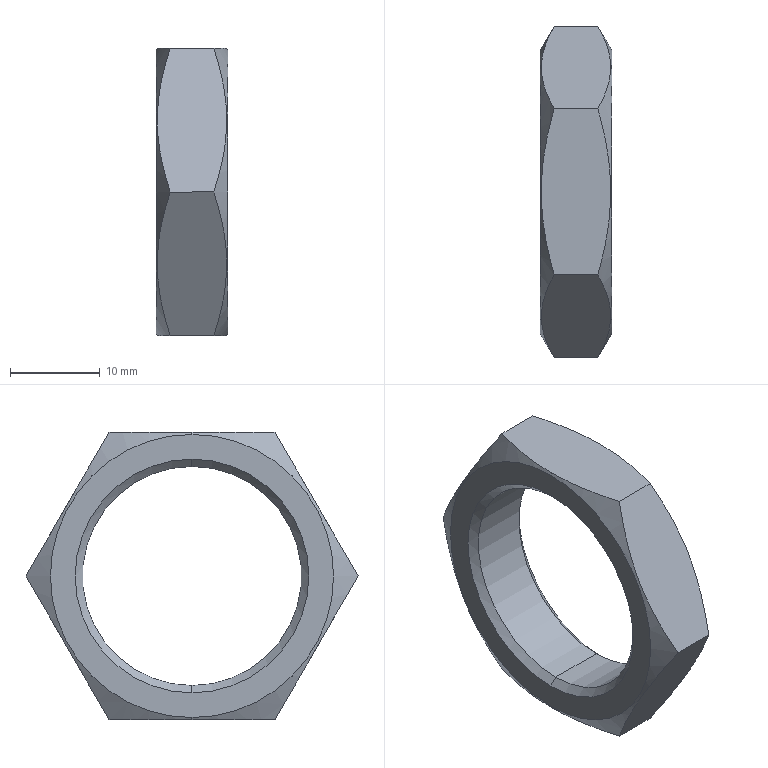Part | SolidWorks | features BaseBody 1 | 1 solid | 18 faces | box 8 x 36.95 x 32 mm | volume 3211 mm3 | cone 8 | plane 8 | cylinder 2 | commonest cylinder face diameters 24.376 x2
STEP:
#1=CARTESIAN_POINT('',(-3.188,0.,12.188));
#2=VERTEX_POINT('',#1);
#3=CARTESIAN_POINT('',(-3.188,0.,-12.188));
#4=VERTEX_POINT('',#3);
#5=CARTESIAN_POINT('',(-3.188,0.,0.));
#6=DIRECTION('',(1.,0.,0.));
#7=DIRECTION('',(0.,0.,-1.));
#8=AXIS2_PLACEMENT_3D('',#5,#6,#7);
#9=CIRCLE('',#8,12.188);
#10=EDGE_CURVE('',#2,#4,#9,.T.);
#11=ORIENTED_EDGE('',*,*,#10,.F.);
#12=CARTESIAN_POINT('',(3.188,0.,12.188));
#13=VERTEX_POINT('',#12);
#14=CARTESIAN_POINT('',(4.,0.,12.188));
#15=DIRECTION('',(1.,0.,0.));
#16=VECTOR('',#15,1000.);
#17=LINE('',#14,#16);
#18=EDGE_CURVE('',#2,#13,#17,.T.);
#19=ORIENTED_EDGE('',*,*,#18,.T.);
#20=CARTESIAN_POINT('',(3.188,0.,-12.188));
#21=VERTEX_POINT('',#20);
#22=CARTESIAN_POINT('',(3.188,0.,0.));
#23=DIRECTION('',(-1.,0.,0.));
#24=DIRECTION('',(0.,0.,-1.));
#25=AXIS2_PLACEMENT_3D('',#22,#23,#24);
#26=CIRCLE('',#25,12.188);
#27=EDGE_CURVE('',#21,#13,#26,.T.);
#28=ORIENTED_EDGE('',*,*,#27,.F.);
#29=CARTESIAN_POINT('',(4.,0.,-12.188));
#30=DIRECTION('',(1.,0.,0.));
#31=VECTOR('',#30,1000.);
#32=LINE('',#29,#31);
#33=EDGE_CURVE('',#4,#21,#32,.T.);
#34=ORIENTED_EDGE('',*,*,#33,.F.);
#35=EDGE_LOOP('',(#11,#19,#28,#34));
#36=FACE_OUTER_BOUND('',#35,.T.);
#37=CARTESIAN_POINT('',(4.,0.,0.));
#38=DIRECTION('',(1.,0.,0.));
#39=DIRECTION('',(0.,0.,-1.));
#40=AXIS2_PLACEMENT_3D('',#37,#38,#39);
#41=CYLINDRICAL_SURFACE('',#40,12.188);
#42=ADVANCED_FACE('',(#36),#41,.F.);
#43=ORIENTED_EDGE('',*,*,#10,.T.);
#44=CARTESIAN_POINT('',(-4.,0.,-13.));
#45=VERTEX_POINT('',#44);
#46=CARTESIAN_POINT('',(-4.,0.,-13.));
#47=DIRECTION('',(-0.7071,0.,-0.7071));
#48=VECTOR('',#47,1000.);
#49=LINE('',#46,#48);
#50=EDGE_CURVE('',#4,#45,#49,.T.);
#51=ORIENTED_EDGE('',*,*,#50,.T.);
#52=CARTESIAN_POINT('',(-4.,0.,13.));
#53=VERTEX_POINT('',#52);
#54=CARTESIAN_POINT('',(-4.,0.,0.));
#55=DIRECTION('',(1.,0.,0.));
#56=DIRECTION('',(0.,0.,1.));
#57=AXIS2_PLACEMENT_3D('',#54,#55,#56);
#58=CIRCLE('',#57,13.);
#59=EDGE_CURVE('',#53,#45,#58,.T.);
#60=ORIENTED_EDGE('',*,*,#59,.F.);
#61=CARTESIAN_POINT('',(-4.,0.,13.));
#62=DIRECTION('',(-0.7071,0.,0.7071));
#63=VECTOR('',#62,1000.);
#64=LINE('',#61,#63);
#65=EDGE_CURVE('',#2,#53,#64,.T.);
#66=ORIENTED_EDGE('',*,*,#65,.F.);
#67=EDGE_LOOP('',(#43,#51,#60,#66));
#68=FACE_OUTER_BOUND('',#67,.T.);
#69=CARTESIAN_POINT('',(-4.,0.,0.));
#70=DIRECTION('',(-1.,0.,0.));
#71=DIRECTION('',(0.,0.,1.));
#72=AXIS2_PLACEMENT_3D('',#69,#70,#71);
#73=CONICAL_SURFACE('',#72,13.,0.7854);
#74=ADVANCED_FACE('',(#68),#73,.F.);
#75=ORIENTED_EDGE('',*,*,#27,.T.);
#76=CARTESIAN_POINT('',(4.,0.,13.));
#77=VERTEX_POINT('',#76);
#78=CARTESIAN_POINT('',(4.,0.,13.));
#79=DIRECTION('',(0.7071,0.,0.7071));
#80=VECTOR('',#79,1000.);
#81=LINE('',#78,#80);
#82=EDGE_CURVE('',#13,#77,#81,.T.);
#83=ORIENTED_EDGE('',*,*,#82,.T.);
#84=CARTESIAN_POINT('',(4.,0.,-13.));
#85=VERTEX_POINT('',#84);
#86=CARTESIAN_POINT('',(4.,0.,0.));
#87=DIRECTION('',(-1.,0.,0.));
#88=DIRECTION('',(0.,0.,-1.));
#89=AXIS2_PLACEMENT_3D('',#86,#87,#88);
#90=CIRCLE('',#89,13.);
#91=EDGE_CURVE('',#85,#77,#90,.T.);
#92=ORIENTED_EDGE('',*,*,#91,.F.);
#93=CARTESIAN_POINT('',(4.,0.,-13.));
#94=DIRECTION('',(0.7071,0.,-0.7071));
#95=VECTOR('',#94,1000.);
#96=LINE('',#93,#95);
#97=EDGE_CURVE('',#21,#85,#96,.T.);
#98=ORIENTED_EDGE('',*,*,#97,.F.);
#99=EDGE_LOOP('',(#75,#83,#92,#98));
#100=FACE_OUTER_BOUND('',#99,.T.);
#101=CARTESIAN_POINT('',(4.,0.,0.));
#102=DIRECTION('',(1.,0.,0.));
#103=DIRECTION('',(0.,0.,-1.));
#104=AXIS2_PLACEMENT_3D('',#101,#102,#103);
#105=CONICAL_SURFACE('',#104,13.,0.7854);
#106=ADVANCED_FACE('',(#100),#105,.F.);
#107=CARTESIAN_POINT('',(-4.,0.,-15.75));
#108=VERTEX_POINT('',#107);
#109=CARTESIAN_POINT('',(-4.,0.,15.75));
#110=VERTEX_POINT('',#109);
#111=CARTESIAN_POINT('',(-4.,0.,0.));
#112=DIRECTION('',(1.,0.,0.));
#113=DIRECTION('',(0.,0.,-1.));
#114=AXIS2_PLACEMENT_3D('',#111,#112,#113);
#115=CIRCLE('',#114,15.75);
#116=EDGE_CURVE('',#108,#110,#115,.T.);
#117=ORIENTED_EDGE('',*,*,#116,.T.);
#118=CARTESIAN_POINT('',(-3.856,0.,16.));
#119=VERTEX_POINT('',#118);
#120=CARTESIAN_POINT('',(-2.417,0.,18.492));
#121=DIRECTION('',(0.5,0.,0.866));
#122=VECTOR('',#121,1000.);
#123=LINE('',#120,#122);
#124=EDGE_CURVE('',#110,#119,#123,.T.);
#125=ORIENTED_EDGE('',*,*,#124,.T.);
#126=CARTESIAN_POINT('',(-2.427,9.238,16.));
#127=VERTEX_POINT('',#126);
#128=CARTESIAN_POINT('',(-3.856,0.,16.));
#129=CARTESIAN_POINT('',(-3.856,0.784,16.));
#130=CARTESIAN_POINT('',(-3.822,1.571,16.));
#131=CARTESIAN_POINT('',(-3.691,3.129,16.));
#132=CARTESIAN_POINT('',(-3.594,3.903,16.));
#133=CARTESIAN_POINT('',(-3.221,6.21,16.));
#134=CARTESIAN_POINT('',(-2.862,7.73,16.));
#135=CARTESIAN_POINT('',(-2.427,9.238,16.));
#136=B_SPLINE_CURVE_WITH_KNOTS('',3,(#128,#129,#130,#131,#132,#133,#134,#135),.UNSPECIFIED.,.F.,.F.,(4,2,2,4),(0.009347,0.01167,0.014,0.01866),.UNSPECIFIED.);
#137=EDGE_CURVE('',#119,#127,#136,.T.);
#138=ORIENTED_EDGE('',*,*,#137,.T.);
#139=CARTESIAN_POINT('',(-2.427,18.475,0.000000043));
#140=VERTEX_POINT('',#139);
#141=CARTESIAN_POINT('',(-2.427,9.238,16.));
#142=CARTESIAN_POINT('',(-2.862,9.992,14.694));
#143=CARTESIAN_POINT('',(-3.221,10.751,13.378));
#144=CARTESIAN_POINT('',(-3.718,12.287,10.719));
#145=CARTESIAN_POINT('',(-3.855,13.062,9.376));
#146=CARTESIAN_POINT('',(-3.856,14.24,7.335));
#147=CARTESIAN_POINT('',(-3.823,14.635,6.652));
#148=CARTESIAN_POINT('',(-3.693,15.415,5.3));
#149=CARTESIAN_POINT('',(-3.596,15.803,4.629));
#150=CARTESIAN_POINT('',(-3.222,16.959,2.627));
#151=CARTESIAN_POINT('',(-2.863,17.72,1.308));
#152=CARTESIAN_POINT('',(-2.427,18.475,0.000000043));
#153=B_SPLINE_CURVE_WITH_KNOTS('',3,(#141,#142,#143,#144,#145,#146,#147,#148,#149,#150,#151,#152),.UNSPECIFIED.,.F.,.F.,(4,2,2,2,2,4),(0.,0.004665,0.009329,0.01166,0.01399,0.01866),.UNSPECIFIED.);
#154=EDGE_CURVE('',#127,#140,#153,.T.);
#155=ORIENTED_EDGE('',*,*,#154,.T.);
#156=CARTESIAN_POINT('',(-2.427,9.238,-16.));
#157=VERTEX_POINT('',#156);
#158=CARTESIAN_POINT('',(-2.427,18.475,0.000000043));
#159=CARTESIAN_POINT('',(-2.862,17.721,-1.306));
#160=CARTESIAN_POINT('',(-3.221,16.961,-2.622));
#161=CARTESIAN_POINT('',(-3.718,15.426,-5.281));
#162=CARTESIAN_POINT('',(-3.855,14.651,-6.624));
#163=CARTESIAN_POINT('',(-3.856,13.473,-8.665));
#164=CARTESIAN_POINT('',(-3.823,13.078,-9.348));
#165=CARTESIAN_POINT('',(-3.693,12.298,-10.7));
#166=CARTESIAN_POINT('',(-3.596,11.91,-11.371));
#167=CARTESIAN_POINT('',(-3.222,10.754,-13.373));
#168=CARTESIAN_POINT('',(-2.863,9.993,-14.692));
#169=CARTESIAN_POINT('',(-2.427,9.238,-16.));
#170=B_SPLINE_CURVE_WITH_KNOTS('',3,(#158,#159,#160,#161,#162,#163,#164,#165,#166,#167,#168,#169),.UNSPECIFIED.,.F.,.F.,(4,2,2,2,2,4),(0.,0.004665,0.009329,0.01166,0.01399,0.01866),.UNSPECIFIED.);
#171=EDGE_CURVE('',#140,#157,#170,.T.);
#172=ORIENTED_EDGE('',*,*,#171,.T.);
#173=CARTESIAN_POINT('',(-3.856,0.,-16.));
#174=VERTEX_POINT('',#173);
#175=CARTESIAN_POINT('',(-2.427,9.238,-16.));
#176=CARTESIAN_POINT('',(-2.863,7.726,-16.));
#177=CARTESIAN_POINT('',(-3.222,6.204,-16.));
#178=CARTESIAN_POINT('',(-3.719,3.128,-16.));
#179=CARTESIAN_POINT('',(-3.856,1.574,-16.));
#180=CARTESIAN_POINT('',(-3.856,0.,-16.));
#181=B_SPLINE_CURVE_WITH_KNOTS('',3,(#175,#176,#177,#178,#179,#180),.UNSPECIFIED.,.F.,.F.,(4,2,4),(0.,0.004673,0.009347),.UNSPECIFIED.);
#182=EDGE_CURVE('',#157,#174,#181,.T.);
#183=ORIENTED_EDGE('',*,*,#182,.T.);
#184=CARTESIAN_POINT('',(-2.417,0.,-18.492));
#185=DIRECTION('',(0.5,0.,-0.866));
#186=VECTOR('',#185,1000.);
#187=LINE('',#184,#186);
#188=EDGE_CURVE('',#108,#174,#187,.T.);
#189=ORIENTED_EDGE('',*,*,#188,.F.);
#190=EDGE_LOOP('',(#117,#125,#138,#155,#172,#183,#189));
#191=FACE_OUTER_BOUND('',#190,.T.);
#192=CARTESIAN_POINT('',(-2.417,0.,0.));
#193=DIRECTION('',(1.,0.,0.));
#194=DIRECTION('',(0.,0.,-1.));
#195=AXIS2_PLACEMENT_3D('',#192,#193,#194);
#196=CONICAL_SURFACE('',#195,18.492,1.047);
#197=ADVANCED_FACE('',(#191),#196,.T.);
#198=CARTESIAN_POINT('',(4.,0.,-15.75));
#199=VERTEX_POINT('',#198);
#200=CARTESIAN_POINT('',(4.,0.,15.75));
#201=VERTEX_POINT('',#200);
#202=CARTESIAN_POINT('',(4.,0.,0.));
#203=DIRECTION('',(1.,0.,0.));
#204=DIRECTION('',(0.,0.,1.));
#205=AXIS2_PLACEMENT_3D('',#202,#203,#204);
#206=CIRCLE('',#205,15.75);
#207=EDGE_CURVE('',#199,#201,#206,.T.);
#208=ORIENTED_EDGE('',*,*,#207,.F.);
#209=CARTESIAN_POINT('',(3.856,0.,-16.));
#210=VERTEX_POINT('',#209);
#211=CARTESIAN_POINT('',(2.417,0.,-18.492));
#212=DIRECTION('',(-0.5,0.,-0.866));
#213=VECTOR('',#212,1000.);
#214=LINE('',#211,#213);
#215=EDGE_CURVE('',#199,#210,#214,.T.);
#216=ORIENTED_EDGE('',*,*,#215,.T.);
#217=CARTESIAN_POINT('',(2.427,9.238,-16.));
#218=VERTEX_POINT('',#217);
#219=CARTESIAN_POINT('',(3.856,0.,-16.));
#220=CARTESIAN_POINT('',(3.856,0.784,-16.));
#221=CARTESIAN_POINT('',(3.822,1.571,-16.));
#222=CARTESIAN_POINT('',(3.691,3.129,-16.));
#223=CARTESIAN_POINT('',(3.594,3.903,-16.));
#224=CARTESIAN_POINT('',(3.221,6.21,-16.));
#225=CARTESIAN_POINT('',(2.862,7.73,-16.));
#226=CARTESIAN_POINT('',(2.427,9.238,-16.));
#227=B_SPLINE_CURVE_WITH_KNOTS('',3,(#219,#220,#221,#222,#223,#224,#225,#226),.UNSPECIFIED.,.F.,.F.,(4,2,2,4),(0.009347,0.01167,0.014,0.01866),.UNSPECIFIED.);
#228=EDGE_CURVE('',#210,#218,#227,.T.);
#229=ORIENTED_EDGE('',*,*,#228,.T.);
#230=CARTESIAN_POINT('',(2.427,18.475,-0.000000043));
#231=VERTEX_POINT('',#230);
#232=CARTESIAN_POINT('',(2.427,9.238,-16.));
#233=CARTESIAN_POINT('',(2.862,9.992,-14.694));
#234=CARTESIAN_POINT('',(3.221,10.751,-13.378));
#235=CARTESIAN_POINT('',(3.718,12.287,-10.719));
#236=CARTESIAN_POINT('',(3.855,13.062,-9.376));
#237=CARTESIAN_POINT('',(3.856,14.24,-7.335));
#238=CARTESIAN_POINT('',(3.823,14.635,-6.652));
#239=CARTESIAN_POINT('',(3.693,15.415,-5.3));
#240=CARTESIAN_POINT('',(3.596,15.803,-4.629));
#241=CARTESIAN_POINT('',(3.222,16.959,-2.627));
#242=CARTESIAN_POINT('',(2.863,17.72,-1.308));
#243=CARTESIAN_POINT('',(2.427,18.475,-0.000000043));
#244=B_SPLINE_CURVE_WITH_KNOTS('',3,(#232,#233,#234,#235,#236,#237,#238,#239,#240,#241,#242,#243),.UNSPECIFIED.,.F.,.F.,(4,2,2,2,2,4),(0.,0.004665,0.009329,0.01166,0.01399,0.01866),.UNSPECIFIED.);
#245=EDGE_CURVE('',#218,#231,#244,.T.);
#246=ORIENTED_EDGE('',*,*,#245,.T.);
#247=CARTESIAN_POINT('',(2.427,9.238,16.));
#248=VERTEX_POINT('',#247);
#249=CARTESIAN_POINT('',(2.427,18.475,-0.000000043));
#250=CARTESIAN_POINT('',(2.862,17.721,1.306));
#251=CARTESIAN_POINT('',(3.221,16.961,2.622));
#252=CARTESIAN_POINT('',(3.718,15.426,5.281));
#253=CARTESIAN_POINT('',(3.855,14.651,6.624));
#254=CARTESIAN_POINT('',(3.856,13.473,8.665));
#255=CARTESIAN_POINT('',(3.823,13.078,9.348));
#256=CARTESIAN_POINT('',(3.693,12.298,10.7));
#257=CARTESIAN_POINT('',(3.596,11.91,11.371));
#258=CARTESIAN_POINT('',(3.222,10.754,13.373));
#259=CARTESIAN_POINT('',(2.863,9.993,14.692));
#260=CARTESIAN_POINT('',(2.427,9.238,16.));
#261=B_SPLINE_CURVE_WITH_KNOTS('',3,(#249,#250,#251,#252,#253,#254,#255,#256,#257,#258,#259,#260),.UNSPECIFIED.,.F.,.F.,(4,2,2,2,2,4),(0.,0.004665,0.009329,0.01166,0.01399,0.01866),.UNSPECIFIED.);
#262=EDGE_CURVE('',#231,#248,#261,.T.);
#263=ORIENTED_EDGE('',*,*,#262,.T.);
#264=CARTESIAN_POINT('',(3.856,0.,16.));
#265=VERTEX_POINT('',#264);
#266=CARTESIAN_POINT('',(2.427,9.238,16.));
#267=CARTESIAN_POINT('',(2.863,7.726,16.));
#268=CARTESIAN_POINT('',(3.222,6.204,16.));
#269=CARTESIAN_POINT('',(3.719,3.128,16.));
#270=CARTESIAN_POINT('',(3.856,1.574,16.));
#271=CARTESIAN_POINT('',(3.856,0.,16.));
#272=B_SPLINE_CURVE_WITH_KNOTS('',3,(#266,#267,#268,#269,#270,#271),.UNSPECIFIED.,.F.,.F.,(4,2,4),(0.,0.004673,0.009347),.UNSPECIFIED.);
#273=EDGE_CURVE('',#248,#265,#272,.T.);
#274=ORIENTED_EDGE('',*,*,#273,.T.);
#275=CARTESIAN_POINT('',(2.417,0.,18.492));
#276=DIRECTION('',(-0.5,0.,0.866));
#277=VECTOR('',#276,1000.);
#278=LINE('',#275,#277);
#279=EDGE_CURVE('',#201,#265,#278,.T.);
#280=ORIENTED_EDGE('',*,*,#279,.F.);
#281=EDGE_LOOP('',(#208,#216,#229,#246,#263,#274,#280));
#282=FACE_OUTER_BOUND('',#281,.T.);
#283=CARTESIAN_POINT('',(2.417,0.,0.));
#284=DIRECTION('',(-1.,0.,0.));
#285=DIRECTION('',(0.,0.,1.));
#286=AXIS2_PLACEMENT_3D('',#283,#284,#285);
#287=CONICAL_SURFACE('',#286,18.492,1.047);
#288=ADVANCED_FACE('',(#282),#287,.T.);
#289=ORIENTED_EDGE('',*,*,#18,.F.);
#290=CARTESIAN_POINT('',(-3.188,0.,0.));
#291=DIRECTION('',(1.,0.,0.));
#292=DIRECTION('',(0.,0.,-1.));
#293=AXIS2_PLACEMENT_3D('',#290,#291,#292);
#294=CIRCLE('',#293,12.188);
#295=EDGE_CURVE('',#4,#2,#294,.T.);
#296=ORIENTED_EDGE('',*,*,#295,.F.);
#297=ORIENTED_EDGE('',*,*,#33,.T.);
#298=CARTESIAN_POINT('',(3.188,0.,0.));
#299=DIRECTION('',(-1.,0.,0.));
#300=DIRECTION('',(0.,0.,-1.));
#301=AXIS2_PLACEMENT_3D('',#298,#299,#300);
#302=CIRCLE('',#301,12.188);
#303=EDGE_CURVE('',#13,#21,#302,.T.);
#304=ORIENTED_EDGE('',*,*,#303,.F.);
#305=EDGE_LOOP('',(#289,#296,#297,#304));
#306=FACE_OUTER_BOUND('',#305,.T.);
#307=CARTESIAN_POINT('',(4.,0.,0.));
#308=DIRECTION('',(1.,0.,0.));
#309=DIRECTION('',(0.,0.,-1.));
#310=AXIS2_PLACEMENT_3D('',#307,#308,#309);
#311=CYLINDRICAL_SURFACE('',#310,12.188);
#312=ADVANCED_FACE('',(#306),#311,.F.);
#313=ORIENTED_EDGE('',*,*,#50,.F.);
#314=ORIENTED_EDGE('',*,*,#295,.T.);
#315=ORIENTED_EDGE('',*,*,#65,.T.);
#316=CARTESIAN_POINT('',(-4.,0.,0.));
#317=DIRECTION('',(1.,0.,0.));
#318=DIRECTION('',(0.,0.,1.));
#319=AXIS2_PLACEMENT_3D('',#316,#317,#318);
#320=CIRCLE('',#319,13.);
#321=EDGE_CURVE('',#45,#53,#320,.T.);
#322=ORIENTED_EDGE('',*,*,#321,.F.);
#323=EDGE_LOOP('',(#313,#314,#315,#322));
#324=FACE_OUTER_BOUND('',#323,.T.);
#325=CARTESIAN_POINT('',(-4.,0.,0.));
#326=DIRECTION('',(-1.,0.,0.));
#327=DIRECTION('',(0.,0.,1.));
#328=AXIS2_PLACEMENT_3D('',#325,#326,#327);
#329=CONICAL_SURFACE('',#328,13.,0.7854);
#330=ADVANCED_FACE('',(#324),#329,.F.);
#331=ORIENTED_EDGE('',*,*,#82,.F.);
#332=ORIENTED_EDGE('',*,*,#303,.T.);
#333=ORIENTED_EDGE('',*,*,#97,.T.);
#334=CARTESIAN_POINT('',(4.,0.,0.));
#335=DIRECTION('',(-1.,0.,0.));
#336=DIRECTION('',(0.,0.,-1.));
#337=AXIS2_PLACEMENT_3D('',#334,#335,#336);
#338=CIRCLE('',#337,13.);
#339=EDGE_CURVE('',#77,#85,#338,.T.);
#340=ORIENTED_EDGE('',*,*,#339,.F.);
#341=EDGE_LOOP('',(#331,#332,#333,#340));
#342=FACE_OUTER_BOUND('',#341,.T.);
#343=CARTESIAN_POINT('',(4.,0.,0.));
#344=DIRECTION('',(1.,0.,0.));
#345=DIRECTION('',(0.,0.,-1.));
#346=AXIS2_PLACEMENT_3D('',#343,#344,#345);
#347=CONICAL_SURFACE('',#346,13.,0.7854);
#348=ADVANCED_FACE('',(#342),#347,.F.);
#349=ORIENTED_EDGE('',*,*,#116,.F.);
#350=CARTESIAN_POINT('',(-4.,0.,0.));
#351=DIRECTION('',(1.,0.,0.));
#352=DIRECTION('',(0.,0.,-1.));
#353=AXIS2_PLACEMENT_3D('',#350,#351,#352);
#354=CIRCLE('',#353,15.75);
#355=EDGE_CURVE('',#110,#108,#354,.T.);
#356=ORIENTED_EDGE('',*,*,#355,.F.);
#357=EDGE_LOOP('',(#349,#356));
#358=FACE_OUTER_BOUND('',#357,.T.);
#359=ORIENTED_EDGE('',*,*,#59,.T.);
#360=ORIENTED_EDGE('',*,*,#321,.T.);
#361=EDGE_LOOP('',(#359,#360));
#362=FACE_BOUND('',#361,.T.);
#363=CARTESIAN_POINT('',(-4.,0.,0.));
#364=DIRECTION('',(1.,0.,0.));
#365=DIRECTION('',(0.,0.,-1.));
#366=AXIS2_PLACEMENT_3D('',#363,#364,#365);
#367=PLANE('',#366);
#368=ADVANCED_FACE('',(#358,#362),#367,.F.);
#369=CARTESIAN_POINT('',(4.,0.,0.));
#370=DIRECTION('',(1.,0.,0.));
#371=DIRECTION('',(0.,0.,1.));
#372=AXIS2_PLACEMENT_3D('',#369,#370,#371);
#373=CIRCLE('',#372,15.75);
#374=EDGE_CURVE('',#201,#199,#373,.T.);
#375=ORIENTED_EDGE('',*,*,#374,.T.);
#376=ORIENTED_EDGE('',*,*,#207,.T.);
#377=EDGE_LOOP('',(#375,#376));
#378=FACE_OUTER_BOUND('',#377,.T.);
#379=ORIENTED_EDGE('',*,*,#91,.T.);
#380=ORIENTED_EDGE('',*,*,#339,.T.);
#381=EDGE_LOOP('',(#379,#380));
#382=FACE_BOUND('',#381,.T.);
#383=CARTESIAN_POINT('',(4.,0.,0.));
#384=DIRECTION('',(1.,0.,0.));
#385=DIRECTION('',(0.,0.,-1.));
#386=AXIS2_PLACEMENT_3D('',#383,#384,#385);
#387=PLANE('',#386);
#388=ADVANCED_FACE('',(#378,#382),#387,.T.);
#389=ORIENTED_EDGE('',*,*,#124,.F.);
#390=ORIENTED_EDGE('',*,*,#355,.T.);
#391=ORIENTED_EDGE('',*,*,#188,.T.);
#392=CARTESIAN_POINT('',(-2.427,-9.238,-16.));
#393=VERTEX_POINT('',#392);
#394=CARTESIAN_POINT('',(-3.856,0.,-16.));
#395=CARTESIAN_POINT('',(-3.856,-0.784,-16.));
#396=CARTESIAN_POINT('',(-3.822,-1.571,-16.));
#397=CARTESIAN_POINT('',(-3.691,-3.129,-16.));
#398=CARTESIAN_POINT('',(-3.594,-3.903,-16.));
#399=CARTESIAN_POINT('',(-3.221,-6.21,-16.));
#400=CARTESIAN_POINT('',(-2.862,-7.73,-16.));
#401=CARTESIAN_POINT('',(-2.427,-9.238,-16.));
#402=B_SPLINE_CURVE_WITH_KNOTS('',3,(#394,#395,#396,#397,#398,#399,#400,#401),.UNSPECIFIED.,.F.,.F.,(4,2,2,4),(0.009347,0.01167,0.014,0.01866),.UNSPECIFIED.);
#403=EDGE_CURVE('',#174,#393,#402,.T.);
#404=ORIENTED_EDGE('',*,*,#403,.T.);
#405=CARTESIAN_POINT('',(-2.427,-18.475,-0.000000043));
#406=VERTEX_POINT('',#405);
#407=CARTESIAN_POINT('',(-2.427,-9.238,-16.));
#408=CARTESIAN_POINT('',(-2.862,-9.992,-14.694));
#409=CARTESIAN_POINT('',(-3.221,-10.751,-13.378));
#410=CARTESIAN_POINT('',(-3.718,-12.287,-10.719));
#411=CARTESIAN_POINT('',(-3.855,-13.062,-9.376));
#412=CARTESIAN_POINT('',(-3.856,-14.24,-7.335));
#413=CARTESIAN_POINT('',(-3.823,-14.635,-6.652));
#414=CARTESIAN_POINT('',(-3.693,-15.415,-5.3));
#415=CARTESIAN_POINT('',(-3.596,-15.803,-4.629));
#416=CARTESIAN_POINT('',(-3.222,-16.959,-2.627));
#417=CARTESIAN_POINT('',(-2.863,-17.72,-1.308));
#418=CARTESIAN_POINT('',(-2.427,-18.475,-0.000000043));
#419=B_SPLINE_CURVE_WITH_KNOTS('',3,(#407,#408,#409,#410,#411,#412,#413,#414,#415,#416,#417,#418),.UNSPECIFIED.,.F.,.F.,(4,2,2,2,2,4),(0.,0.004665,0.009329,0.01166,0.01399,0.01866),.UNSPECIFIED.);
#420=EDGE_CURVE('',#393,#406,#419,.T.);
#421=ORIENTED_EDGE('',*,*,#420,.T.);
#422=CARTESIAN_POINT('',(-2.427,-9.238,16.));
#423=VERTEX_POINT('',#422);
#424=CARTESIAN_POINT('',(-2.427,-18.475,-0.000000043));
#425=CARTESIAN_POINT('',(-2.862,-17.721,1.306));
#426=CARTESIAN_POINT('',(-3.221,-16.961,2.622));
#427=CARTESIAN_POINT('',(-3.718,-15.426,5.281));
#428=CARTESIAN_POINT('',(-3.855,-14.651,6.624));
#429=CARTESIAN_POINT('',(-3.856,-13.473,8.665));
#430=CARTESIAN_POINT('',(-3.823,-13.078,9.348));
#431=CARTESIAN_POINT('',(-3.693,-12.298,10.7));
#432=CARTESIAN_POINT('',(-3.596,-11.91,11.371));
#433=CARTESIAN_POINT('',(-3.222,-10.754,13.373));
#434=CARTESIAN_POINT('',(-2.863,-9.993,14.692));
#435=CARTESIAN_POINT('',(-2.427,-9.238,16.));
#436=B_SPLINE_CURVE_WITH_KNOTS('',3,(#424,#425,#426,#427,#428,#429,#430,#431,#432,#433,#434,#435),.UNSPECIFIED.,.F.,.F.,(4,2,2,2,2,4),(0.,0.004665,0.009329,0.01166,0.01399,0.01866),.UNSPECIFIED.);
#437=EDGE_CURVE('',#406,#423,#436,.T.);
#438=ORIENTED_EDGE('',*,*,#437,.T.);
#439=CARTESIAN_POINT('',(-2.427,-9.238,16.));
#440=CARTESIAN_POINT('',(-2.863,-7.726,16.));
#441=CARTESIAN_POINT('',(-3.222,-6.204,16.));
#442=CARTESIAN_POINT('',(-3.719,-3.128,16.));
#443=CARTESIAN_POINT('',(-3.856,-1.574,16.));
#444=CARTESIAN_POINT('',(-3.856,0.,16.));
#445=B_SPLINE_CURVE_WITH_KNOTS('',3,(#439,#440,#441,#442,#443,#444),.UNSPECIFIED.,.F.,.F.,(4,2,4),(0.,0.004673,0.009347),.UNSPECIFIED.);
#446=EDGE_CURVE('',#423,#119,#445,.T.);
#447=ORIENTED_EDGE('',*,*,#446,.T.);
#448=EDGE_LOOP('',(#389,#390,#391,#404,#421,#438,#447));
#449=FACE_OUTER_BOUND('',#448,.T.);
#450=CARTESIAN_POINT('',(-2.417,0.,0.));
#451=DIRECTION('',(1.,0.,0.));
#452=DIRECTION('',(0.,0.,-1.));
#453=AXIS2_PLACEMENT_3D('',#450,#451,#452);
#454=CONICAL_SURFACE('',#453,18.492,1.047);
#455=ADVANCED_FACE('',(#449),#454,.T.);
#456=ORIENTED_EDGE('',*,*,#215,.F.);
#457=ORIENTED_EDGE('',*,*,#374,.F.);
#458=ORIENTED_EDGE('',*,*,#279,.T.);
#459=CARTESIAN_POINT('',(2.427,-9.238,16.));
#460=VERTEX_POINT('',#459);
#461=CARTESIAN_POINT('',(3.856,0.,16.));
#462=CARTESIAN_POINT('',(3.856,-0.784,16.));
#463=CARTESIAN_POINT('',(3.822,-1.571,16.));
#464=CARTESIAN_POINT('',(3.691,-3.129,16.));
#465=CARTESIAN_POINT('',(3.594,-3.903,16.));
#466=CARTESIAN_POINT('',(3.221,-6.21,16.));
#467=CARTESIAN_POINT('',(2.862,-7.73,16.));
#468=CARTESIAN_POINT('',(2.427,-9.238,16.));
#469=B_SPLINE_CURVE_WITH_KNOTS('',3,(#461,#462,#463,#464,#465,#466,#467,#468),.UNSPECIFIED.,.F.,.F.,(4,2,2,4),(0.009347,0.01167,0.014,0.01866),.UNSPECIFIED.);
#470=EDGE_CURVE('',#265,#460,#469,.T.);
#471=ORIENTED_EDGE('',*,*,#470,.T.);
#472=CARTESIAN_POINT('',(2.427,-18.475,0.000000043));
#473=VERTEX_POINT('',#472);
#474=CARTESIAN_POINT('',(2.427,-9.238,16.));
#475=CARTESIAN_POINT('',(2.862,-9.992,14.694));
#476=CARTESIAN_POINT('',(3.221,-10.751,13.378));
#477=CARTESIAN_POINT('',(3.718,-12.287,10.719));
#478=CARTESIAN_POINT('',(3.855,-13.062,9.376));
#479=CARTESIAN_POINT('',(3.856,-14.24,7.335));
#480=CARTESIAN_POINT('',(3.823,-14.635,6.652));
#481=CARTESIAN_POINT('',(3.693,-15.415,5.3));
#482=CARTESIAN_POINT('',(3.596,-15.803,4.629));
#483=CARTESIAN_POINT('',(3.222,-16.959,2.627));
#484=CARTESIAN_POINT('',(2.863,-17.72,1.308));
#485=CARTESIAN_POINT('',(2.427,-18.475,0.000000043));
#486=B_SPLINE_CURVE_WITH_KNOTS('',3,(#474,#475,#476,#477,#478,#479,#480,#481,#482,#483,#484,#485),.UNSPECIFIED.,.F.,.F.,(4,2,2,2,2,4),(0.,0.004665,0.009329,0.01166,0.01399,0.01866),.UNSPECIFIED.);
#487=EDGE_CURVE('',#460,#473,#486,.T.);
#488=ORIENTED_EDGE('',*,*,#487,.T.);
#489=CARTESIAN_POINT('',(2.427,-9.238,-16.));
#490=VERTEX_POINT('',#489);
#491=CARTESIAN_POINT('',(2.427,-18.475,0.000000043));
#492=CARTESIAN_POINT('',(2.862,-17.721,-1.306));
#493=CARTESIAN_POINT('',(3.221,-16.961,-2.622));
#494=CARTESIAN_POINT('',(3.718,-15.426,-5.281));
#495=CARTESIAN_POINT('',(3.855,-14.651,-6.624));
#496=CARTESIAN_POINT('',(3.856,-13.473,-8.665));
#497=CARTESIAN_POINT('',(3.823,-13.078,-9.348));
#498=CARTESIAN_POINT('',(3.693,-12.298,-10.7));
#499=CARTESIAN_POINT('',(3.596,-11.91,-11.371));
#500=CARTESIAN_POINT('',(3.222,-10.754,-13.373));
#501=CARTESIAN_POINT('',(2.863,-9.993,-14.692));
#502=CARTESIAN_POINT('',(2.427,-9.238,-16.));
#503=B_SPLINE_CURVE_WITH_KNOTS('',3,(#491,#492,#493,#494,#495,#496,#497,#498,#499,#500,#501,#502),.UNSPECIFIED.,.F.,.F.,(4,2,2,2,2,4),(0.,0.004665,0.009329,0.01166,0.01399,0.01866),.UNSPECIFIED.);
#504=EDGE_CURVE('',#473,#490,#503,.T.);
#505=ORIENTED_EDGE('',*,*,#504,.T.);
#506=CARTESIAN_POINT('',(2.427,-9.238,-16.));
#507=CARTESIAN_POINT('',(2.863,-7.726,-16.));
#508=CARTESIAN_POINT('',(3.222,-6.204,-16.));
#509=CARTESIAN_POINT('',(3.719,-3.128,-16.));
#510=CARTESIAN_POINT('',(3.856,-1.574,-16.));
#511=CARTESIAN_POINT('',(3.856,0.,-16.));
#512=B_SPLINE_CURVE_WITH_KNOTS('',3,(#506,#507,#508,#509,#510,#511),.UNSPECIFIED.,.F.,.F.,(4,2,4),(0.,0.004673,0.009347),.UNSPECIFIED.);
#513=EDGE_CURVE('',#490,#210,#512,.T.);
#514=ORIENTED_EDGE('',*,*,#513,.T.);
#515=EDGE_LOOP('',(#456,#457,#458,#471,#488,#505,#514));
#516=FACE_OUTER_BOUND('',#515,.T.);
#517=CARTESIAN_POINT('',(2.417,0.,0.));
#518=DIRECTION('',(-1.,0.,0.));
#519=DIRECTION('',(0.,0.,1.));
#520=AXIS2_PLACEMENT_3D('',#517,#518,#519);
#521=CONICAL_SURFACE('',#520,18.492,1.047);
#522=ADVANCED_FACE('',(#516),#521,.T.);
#523=ORIENTED_EDGE('',*,*,#446,.F.);
#524=CARTESIAN_POINT('',(4.,-9.238,16.));
#525=DIRECTION('',(-1.,0.,0.));
#526=VECTOR('',#525,1000.);
#527=LINE('',#524,#526);
#528=EDGE_CURVE('',#460,#423,#527,.T.);
#529=ORIENTED_EDGE('',*,*,#528,.F.);
#530=ORIENTED_EDGE('',*,*,#470,.F.);
#531=ORIENTED_EDGE('',*,*,#273,.F.);
#532=CARTESIAN_POINT('',(4.,9.238,16.));
#533=DIRECTION('',(1.,0.,0.));
#534=VECTOR('',#533,1000.);
#535=LINE('',#532,#534);
#536=EDGE_CURVE('',#127,#248,#535,.T.);
#537=ORIENTED_EDGE('',*,*,#536,.F.);
#538=ORIENTED_EDGE('',*,*,#137,.F.);
#539=EDGE_LOOP('',(#523,#529,#530,#531,#537,#538));
#540=FACE_OUTER_BOUND('',#539,.T.);
#541=CARTESIAN_POINT('',(4.,9.238,16.));
#542=DIRECTION('',(0.,0.,-1.));
#543=DIRECTION('',(-1.,0.,0.));
#544=AXIS2_PLACEMENT_3D('',#541,#542,#543);
#545=PLANE('',#544);
#546=ADVANCED_FACE('',(#540),#545,.F.);
#547=ORIENTED_EDGE('',*,*,#437,.F.);
#548=CARTESIAN_POINT('',(4.,-18.475,0.));
#549=DIRECTION('',(-1.,0.,0.));
#550=VECTOR('',#549,1000.);
#551=LINE('',#548,#550);
#552=EDGE_CURVE('',#473,#406,#551,.T.);
#553=ORIENTED_EDGE('',*,*,#552,.F.);
#554=ORIENTED_EDGE('',*,*,#487,.F.);
#555=ORIENTED_EDGE('',*,*,#528,.T.);
#556=EDGE_LOOP('',(#547,#553,#554,#555));
#557=FACE_OUTER_BOUND('',#556,.T.);
#558=CARTESIAN_POINT('',(4.,-9.238,16.));
#559=DIRECTION('',(0.,0.866,-0.5));
#560=DIRECTION('',(0.,0.5,0.866));
#561=AXIS2_PLACEMENT_3D('',#558,#559,#560);
#562=PLANE('',#561);
#563=ADVANCED_FACE('',(#557),#562,.F.);
#564=ORIENTED_EDGE('',*,*,#420,.F.);
#565=CARTESIAN_POINT('',(4.,-9.238,-16.));
#566=DIRECTION('',(-1.,0.,0.));
#567=VECTOR('',#566,1000.);
#568=LINE('',#565,#567);
#569=EDGE_CURVE('',#490,#393,#568,.T.);
#570=ORIENTED_EDGE('',*,*,#569,.F.);
#571=ORIENTED_EDGE('',*,*,#504,.F.);
#572=ORIENTED_EDGE('',*,*,#552,.T.);
#573=EDGE_LOOP('',(#564,#570,#571,#572));
#574=FACE_OUTER_BOUND('',#573,.T.);
#575=CARTESIAN_POINT('',(4.,-18.475,0.));
#576=DIRECTION('',(0.,0.866,0.5));
#577=DIRECTION('',(0.,-0.5,0.866));
#578=AXIS2_PLACEMENT_3D('',#575,#576,#577);
#579=PLANE('',#578);
#580=ADVANCED_FACE('',(#574),#579,.F.);
#581=ORIENTED_EDGE('',*,*,#182,.F.);
#582=CARTESIAN_POINT('',(4.,9.238,-16.));
#583=DIRECTION('',(-1.,0.,0.));
#584=VECTOR('',#583,1000.);
#585=LINE('',#582,#584);
#586=EDGE_CURVE('',#218,#157,#585,.T.);
#587=ORIENTED_EDGE('',*,*,#586,.F.);
#588=ORIENTED_EDGE('',*,*,#228,.F.);
#589=ORIENTED_EDGE('',*,*,#513,.F.);
#590=ORIENTED_EDGE('',*,*,#569,.T.);
#591=ORIENTED_EDGE('',*,*,#403,.F.);
#592=EDGE_LOOP('',(#581,#587,#588,#589,#590,#591));
#593=FACE_OUTER_BOUND('',#592,.T.);
#594=CARTESIAN_POINT('',(4.,-9.238,-16.));
#595=DIRECTION('',(0.,0.,1.));
#596=DIRECTION('',(1.,0.,0.));
#597=AXIS2_PLACEMENT_3D('',#594,#595,#596);
#598=PLANE('',#597);
#599=ADVANCED_FACE('',(#593),#598,.F.);
#600=ORIENTED_EDGE('',*,*,#171,.F.);
#601=CARTESIAN_POINT('',(4.,18.475,0.));
#602=DIRECTION('',(-1.,0.,0.));
#603=VECTOR('',#602,1000.);
#604=LINE('',#601,#603);
#605=EDGE_CURVE('',#231,#140,#604,.T.);
#606=ORIENTED_EDGE('',*,*,#605,.F.);
#607=ORIENTED_EDGE('',*,*,#245,.F.);
#608=ORIENTED_EDGE('',*,*,#586,.T.);
#609=EDGE_LOOP('',(#600,#606,#607,#608));
#610=FACE_OUTER_BOUND('',#609,.T.);
#611=CARTESIAN_POINT('',(4.,9.238,-16.));
#612=DIRECTION('',(0.,-0.866,0.5));
#613=DIRECTION('',(0.,-0.5,-0.866));
#614=AXIS2_PLACEMENT_3D('',#611,#612,#613);
#615=PLANE('',#614);
#616=ADVANCED_FACE('',(#610),#615,.F.);
#617=ORIENTED_EDGE('',*,*,#154,.F.);
#618=ORIENTED_EDGE('',*,*,#536,.T.);
#619=ORIENTED_EDGE('',*,*,#262,.F.);
#620=ORIENTED_EDGE('',*,*,#605,.T.);
#621=EDGE_LOOP('',(#617,#618,#619,#620));
#622=FACE_OUTER_BOUND('',#621,.T.);
#623=CARTESIAN_POINT('',(4.,18.475,0.));
#624=DIRECTION('',(0.,-0.866,-0.5));
#625=DIRECTION('',(0.,0.5,-0.866));
#626=AXIS2_PLACEMENT_3D('',#623,#624,#625);
#627=PLANE('',#626);
#628=ADVANCED_FACE('',(#622),#627,.F.);
#629=CLOSED_SHELL('',(#42,#74,#106,#197,#288,#312,#330,#348,#368,#388,#455,#522,#546,#563,#580,#599,#616,#628));
#630=MANIFOLD_SOLID_BREP('',#629);
#631=CARTESIAN_POINT('',(0.,0.,0.));
#632=DIRECTION('',(0.,0.,1.));
#633=DIRECTION('',(1.,0.,0.));
#634=AXIS2_PLACEMENT_3D('',#631,#632,#633);
#635=(LENGTH_UNIT()NAMED_UNIT(*)SI_UNIT(.MILLI.,.METRE.));
#636=UNCERTAINTY_MEASURE_WITH_UNIT(LENGTH_MEASURE(0.00001),#635,'','');
#637=(NAMED_UNIT(*)PLANE_ANGLE_UNIT()SI_UNIT($,.RADIAN.));
#638=(NAMED_UNIT(*)SI_UNIT($,.STERADIAN.)SOLID_ANGLE_UNIT());
#639=(GEOMETRIC_REPRESENTATION_CONTEXT(3)GLOBAL_UNCERTAINTY_ASSIGNED_CONTEXT((#636))GLOBAL_UNIT_ASSIGNED_CONTEXT((#635,#637,#638))REPRESENTATION_CONTEXT('',''));
#640=ADVANCED_BREP_SHAPE_REPRESENTATION('',(#630,#634),#639);